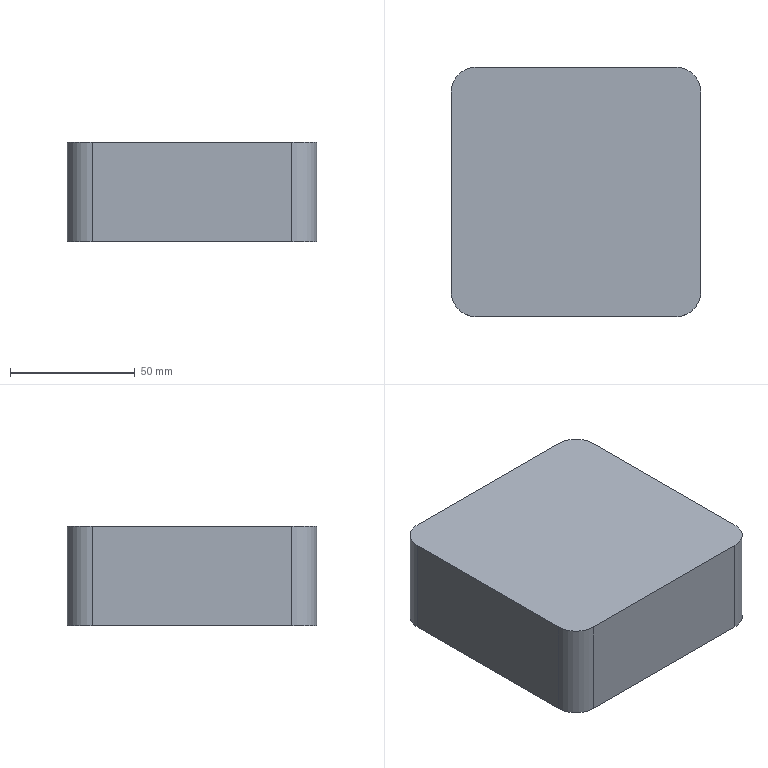Part | SolidWorks | features Extrusion 1, Fillet 1, ICE 1 | 1 solid | 13 faces | box 100 x 100 x 40 mm | volume 264030 mm3 | plane 7 | cylinder 6 | commonest cylinder face diameters 20 x4 75 x2
STEP:
#1=CARTESIAN_POINT('',(37.5,0.,30.));
#2=VERTEX_POINT('',#1);
#3=CARTESIAN_POINT('',(-37.5,0.,30.));
#4=VERTEX_POINT('',#3);
#5=CARTESIAN_POINT('',(0.,0.,30.));
#6=DIRECTION('',(0.,0.,-1.));
#7=DIRECTION('',(-1.,0.,0.));
#8=AXIS2_PLACEMENT_3D('',#5,#6,#7);
#9=CIRCLE('',#8,37.5);
#10=EDGE_CURVE('',#2,#4,#9,.T.);
#11=ORIENTED_EDGE('',*,*,#10,.F.);
#12=CARTESIAN_POINT('',(37.5,0.,0.));
#13=VERTEX_POINT('',#12);
#14=CARTESIAN_POINT('',(37.5,0.,30.));
#15=DIRECTION('',(0.,0.,-1.));
#16=VECTOR('',#15,1000.);
#17=LINE('',#14,#16);
#18=EDGE_CURVE('',#2,#13,#17,.T.);
#19=ORIENTED_EDGE('',*,*,#18,.T.);
#20=CARTESIAN_POINT('',(-37.5,0.,0.));
#21=VERTEX_POINT('',#20);
#22=CARTESIAN_POINT('',(0.,0.,0.));
#23=DIRECTION('',(0.,0.,-1.));
#24=DIRECTION('',(-1.,0.,0.));
#25=AXIS2_PLACEMENT_3D('',#22,#23,#24);
#26=CIRCLE('',#25,37.5);
#27=EDGE_CURVE('',#13,#21,#26,.T.);
#28=ORIENTED_EDGE('',*,*,#27,.T.);
#29=CARTESIAN_POINT('',(-37.5,0.,30.));
#30=DIRECTION('',(0.,0.,-1.));
#31=VECTOR('',#30,1000.);
#32=LINE('',#29,#31);
#33=EDGE_CURVE('',#4,#21,#32,.T.);
#34=ORIENTED_EDGE('',*,*,#33,.F.);
#35=EDGE_LOOP('',(#11,#19,#28,#34));
#36=FACE_OUTER_BOUND('',#35,.T.);
#37=CARTESIAN_POINT('',(0.,0.,30.));
#38=DIRECTION('',(0.,0.,-1.));
#39=DIRECTION('',(-1.,0.,0.));
#40=AXIS2_PLACEMENT_3D('',#37,#38,#39);
#41=CYLINDRICAL_SURFACE('',#40,37.5);
#42=ADVANCED_FACE('',(#36),#41,.F.);
#43=CARTESIAN_POINT('',(-40.,-50.,0.));
#44=VERTEX_POINT('',#43);
#45=CARTESIAN_POINT('',(40.,-50.,0.));
#46=VERTEX_POINT('',#45);
#47=CARTESIAN_POINT('',(-50.,-50.,0.));
#48=DIRECTION('',(1.,0.,0.));
#49=VECTOR('',#48,1000.);
#50=LINE('',#47,#49);
#51=EDGE_CURVE('',#44,#46,#50,.T.);
#52=ORIENTED_EDGE('',*,*,#51,.T.);
#53=CARTESIAN_POINT('',(40.,-50.,40.));
#54=VERTEX_POINT('',#53);
#55=CARTESIAN_POINT('',(40.,-50.,40.));
#56=DIRECTION('',(0.,0.,1.));
#57=VECTOR('',#56,1000.);
#58=LINE('',#55,#57);
#59=EDGE_CURVE('',#46,#54,#58,.T.);
#60=ORIENTED_EDGE('',*,*,#59,.T.);
#61=CARTESIAN_POINT('',(-40.,-50.,40.));
#62=VERTEX_POINT('',#61);
#63=CARTESIAN_POINT('',(-50.,-50.,40.));
#64=DIRECTION('',(1.,0.,0.));
#65=VECTOR('',#64,1000.);
#66=LINE('',#63,#65);
#67=EDGE_CURVE('',#62,#54,#66,.T.);
#68=ORIENTED_EDGE('',*,*,#67,.F.);
#69=CARTESIAN_POINT('',(-40.,-50.,0.));
#70=DIRECTION('',(0.,0.,-1.));
#71=VECTOR('',#70,1000.);
#72=LINE('',#69,#71);
#73=EDGE_CURVE('',#62,#44,#72,.T.);
#74=ORIENTED_EDGE('',*,*,#73,.T.);
#75=EDGE_LOOP('',(#52,#60,#68,#74));
#76=FACE_OUTER_BOUND('',#75,.T.);
#77=CARTESIAN_POINT('',(-50.,-50.,40.));
#78=DIRECTION('',(0.,1.,0.));
#79=DIRECTION('',(0.,0.,1.));
#80=AXIS2_PLACEMENT_3D('',#77,#78,#79);
#81=PLANE('',#80);
#82=ADVANCED_FACE('',(#76),#81,.F.);
#83=CARTESIAN_POINT('',(50.,-40.,40.));
#84=VERTEX_POINT('',#83);
#85=CARTESIAN_POINT('',(50.,40.,40.));
#86=VERTEX_POINT('',#85);
#87=CARTESIAN_POINT('',(50.,-50.,40.));
#88=DIRECTION('',(0.,1.,0.));
#89=VECTOR('',#88,1000.);
#90=LINE('',#87,#89);
#91=EDGE_CURVE('',#84,#86,#90,.T.);
#92=ORIENTED_EDGE('',*,*,#91,.F.);
#93=CARTESIAN_POINT('',(50.,-40.,0.));
#94=VERTEX_POINT('',#93);
#95=CARTESIAN_POINT('',(50.,-40.,40.));
#96=DIRECTION('',(0.,0.,-1.));
#97=VECTOR('',#96,1000.);
#98=LINE('',#95,#97);
#99=EDGE_CURVE('',#84,#94,#98,.T.);
#100=ORIENTED_EDGE('',*,*,#99,.T.);
#101=CARTESIAN_POINT('',(50.,40.,0.));
#102=VERTEX_POINT('',#101);
#103=CARTESIAN_POINT('',(50.,-50.,0.));
#104=DIRECTION('',(0.,1.,0.));
#105=VECTOR('',#104,1000.);
#106=LINE('',#103,#105);
#107=EDGE_CURVE('',#94,#102,#106,.T.);
#108=ORIENTED_EDGE('',*,*,#107,.T.);
#109=CARTESIAN_POINT('',(50.,40.,40.));
#110=DIRECTION('',(0.,0.,1.));
#111=VECTOR('',#110,1000.);
#112=LINE('',#109,#111);
#113=EDGE_CURVE('',#102,#86,#112,.T.);
#114=ORIENTED_EDGE('',*,*,#113,.T.);
#115=EDGE_LOOP('',(#92,#100,#108,#114));
#116=FACE_OUTER_BOUND('',#115,.T.);
#117=CARTESIAN_POINT('',(50.,-50.,40.));
#118=DIRECTION('',(-1.,0.,0.));
#119=DIRECTION('',(0.,0.,1.));
#120=AXIS2_PLACEMENT_3D('',#117,#118,#119);
#121=PLANE('',#120);
#122=ADVANCED_FACE('',(#116),#121,.F.);
#123=CARTESIAN_POINT('',(-40.,50.,40.));
#124=VERTEX_POINT('',#123);
#125=CARTESIAN_POINT('',(40.,50.,40.));
#126=VERTEX_POINT('',#125);
#127=CARTESIAN_POINT('',(-50.,50.,40.));
#128=DIRECTION('',(1.,0.,0.));
#129=VECTOR('',#128,1000.);
#130=LINE('',#127,#129);
#131=EDGE_CURVE('',#124,#126,#130,.T.);
#132=ORIENTED_EDGE('',*,*,#131,.T.);
#133=CARTESIAN_POINT('',(40.,50.,0.));
#134=VERTEX_POINT('',#133);
#135=CARTESIAN_POINT('',(40.,50.,0.));
#136=DIRECTION('',(0.,0.,-1.));
#137=VECTOR('',#136,1000.);
#138=LINE('',#135,#137);
#139=EDGE_CURVE('',#126,#134,#138,.T.);
#140=ORIENTED_EDGE('',*,*,#139,.T.);
#141=CARTESIAN_POINT('',(-40.,50.,0.));
#142=VERTEX_POINT('',#141);
#143=CARTESIAN_POINT('',(-50.,50.,0.));
#144=DIRECTION('',(1.,0.,0.));
#145=VECTOR('',#144,1000.);
#146=LINE('',#143,#145);
#147=EDGE_CURVE('',#142,#134,#146,.T.);
#148=ORIENTED_EDGE('',*,*,#147,.F.);
#149=CARTESIAN_POINT('',(-40.,50.,40.));
#150=DIRECTION('',(0.,0.,1.));
#151=VECTOR('',#150,1000.);
#152=LINE('',#149,#151);
#153=EDGE_CURVE('',#142,#124,#152,.T.);
#154=ORIENTED_EDGE('',*,*,#153,.T.);
#155=EDGE_LOOP('',(#132,#140,#148,#154));
#156=FACE_OUTER_BOUND('',#155,.T.);
#157=CARTESIAN_POINT('',(-50.,50.,40.));
#158=DIRECTION('',(0.,1.,0.));
#159=DIRECTION('',(0.,0.,1.));
#160=AXIS2_PLACEMENT_3D('',#157,#158,#159);
#161=PLANE('',#160);
#162=ADVANCED_FACE('',(#156),#161,.T.);
#163=CARTESIAN_POINT('',(-50.,-40.,0.));
#164=VERTEX_POINT('',#163);
#165=CARTESIAN_POINT('',(-50.,40.,0.));
#166=VERTEX_POINT('',#165);
#167=CARTESIAN_POINT('',(-50.,-50.,0.));
#168=DIRECTION('',(0.,1.,0.));
#169=VECTOR('',#168,1000.);
#170=LINE('',#167,#169);
#171=EDGE_CURVE('',#164,#166,#170,.T.);
#172=ORIENTED_EDGE('',*,*,#171,.F.);
#173=CARTESIAN_POINT('',(-50.,-40.,40.));
#174=VERTEX_POINT('',#173);
#175=CARTESIAN_POINT('',(-50.,-40.,40.));
#176=DIRECTION('',(0.,0.,1.));
#177=VECTOR('',#176,1000.);
#178=LINE('',#175,#177);
#179=EDGE_CURVE('',#164,#174,#178,.T.);
#180=ORIENTED_EDGE('',*,*,#179,.T.);
#181=CARTESIAN_POINT('',(-50.,40.,40.));
#182=VERTEX_POINT('',#181);
#183=CARTESIAN_POINT('',(-50.,-50.,40.));
#184=DIRECTION('',(0.,1.,0.));
#185=VECTOR('',#184,1000.);
#186=LINE('',#183,#185);
#187=EDGE_CURVE('',#174,#182,#186,.T.);
#188=ORIENTED_EDGE('',*,*,#187,.T.);
#189=CARTESIAN_POINT('',(-50.,40.,40.));
#190=DIRECTION('',(0.,0.,-1.));
#191=VECTOR('',#190,1000.);
#192=LINE('',#189,#191);
#193=EDGE_CURVE('',#182,#166,#192,.T.);
#194=ORIENTED_EDGE('',*,*,#193,.T.);
#195=EDGE_LOOP('',(#172,#180,#188,#194));
#196=FACE_OUTER_BOUND('',#195,.T.);
#197=CARTESIAN_POINT('',(-50.,-50.,40.));
#198=DIRECTION('',(-1.,0.,0.));
#199=DIRECTION('',(0.,0.,1.));
#200=AXIS2_PLACEMENT_3D('',#197,#198,#199);
#201=PLANE('',#200);
#202=ADVANCED_FACE('',(#196),#201,.T.);
#203=ORIENTED_EDGE('',*,*,#67,.T.);
#204=CARTESIAN_POINT('',(40.,-40.,40.));
#205=DIRECTION('',(0.,0.,1.));
#206=DIRECTION('',(1.,0.,0.));
#207=AXIS2_PLACEMENT_3D('',#204,#205,#206);
#208=CIRCLE('',#207,10.);
#209=EDGE_CURVE('',#54,#84,#208,.T.);
#210=ORIENTED_EDGE('',*,*,#209,.T.);
#211=ORIENTED_EDGE('',*,*,#91,.T.);
#212=CARTESIAN_POINT('',(40.,40.,40.));
#213=DIRECTION('',(0.,0.,1.));
#214=DIRECTION('',(1.,0.,0.));
#215=AXIS2_PLACEMENT_3D('',#212,#213,#214);
#216=CIRCLE('',#215,10.);
#217=EDGE_CURVE('',#86,#126,#216,.T.);
#218=ORIENTED_EDGE('',*,*,#217,.T.);
#219=ORIENTED_EDGE('',*,*,#131,.F.);
#220=CARTESIAN_POINT('',(-40.,40.,40.));
#221=DIRECTION('',(0.,0.,1.));
#222=DIRECTION('',(1.,0.,0.));
#223=AXIS2_PLACEMENT_3D('',#220,#221,#222);
#224=CIRCLE('',#223,10.);
#225=EDGE_CURVE('',#124,#182,#224,.T.);
#226=ORIENTED_EDGE('',*,*,#225,.T.);
#227=ORIENTED_EDGE('',*,*,#187,.F.);
#228=CARTESIAN_POINT('',(-40.,-40.,40.));
#229=DIRECTION('',(0.,0.,1.));
#230=DIRECTION('',(1.,0.,0.));
#231=AXIS2_PLACEMENT_3D('',#228,#229,#230);
#232=CIRCLE('',#231,10.);
#233=EDGE_CURVE('',#174,#62,#232,.T.);
#234=ORIENTED_EDGE('',*,*,#233,.T.);
#235=EDGE_LOOP('',(#203,#210,#211,#218,#219,#226,#227,#234));
#236=FACE_OUTER_BOUND('',#235,.T.);
#237=CARTESIAN_POINT('',(0.,0.,40.));
#238=DIRECTION('',(0.,0.,1.));
#239=DIRECTION('',(1.,0.,0.));
#240=AXIS2_PLACEMENT_3D('',#237,#238,#239);
#241=PLANE('',#240);
#242=ADVANCED_FACE('',(#236),#241,.T.);
#243=CARTESIAN_POINT('',(0.,0.,0.));
#244=DIRECTION('',(0.,0.,-1.));
#245=DIRECTION('',(-1.,0.,0.));
#246=AXIS2_PLACEMENT_3D('',#243,#244,#245);
#247=CIRCLE('',#246,37.5);
#248=EDGE_CURVE('',#21,#13,#247,.T.);
#249=ORIENTED_EDGE('',*,*,#248,.F.);
#250=ORIENTED_EDGE('',*,*,#27,.F.);
#251=EDGE_LOOP('',(#249,#250));
#252=FACE_BOUND('',#251,.T.);
#253=ORIENTED_EDGE('',*,*,#107,.F.);
#254=CARTESIAN_POINT('',(40.,-40.,0.));
#255=DIRECTION('',(0.,0.,-1.));
#256=DIRECTION('',(1.,0.,0.));
#257=AXIS2_PLACEMENT_3D('',#254,#255,#256);
#258=CIRCLE('',#257,10.);
#259=EDGE_CURVE('',#94,#46,#258,.T.);
#260=ORIENTED_EDGE('',*,*,#259,.T.);
#261=ORIENTED_EDGE('',*,*,#51,.F.);
#262=CARTESIAN_POINT('',(-40.,-40.,0.));
#263=DIRECTION('',(0.,0.,-1.));
#264=DIRECTION('',(1.,0.,0.));
#265=AXIS2_PLACEMENT_3D('',#262,#263,#264);
#266=CIRCLE('',#265,10.);
#267=EDGE_CURVE('',#44,#164,#266,.T.);
#268=ORIENTED_EDGE('',*,*,#267,.T.);
#269=ORIENTED_EDGE('',*,*,#171,.T.);
#270=CARTESIAN_POINT('',(-40.,40.,0.));
#271=DIRECTION('',(0.,0.,-1.));
#272=DIRECTION('',(1.,0.,0.));
#273=AXIS2_PLACEMENT_3D('',#270,#271,#272);
#274=CIRCLE('',#273,10.);
#275=EDGE_CURVE('',#166,#142,#274,.T.);
#276=ORIENTED_EDGE('',*,*,#275,.T.);
#277=ORIENTED_EDGE('',*,*,#147,.T.);
#278=CARTESIAN_POINT('',(40.,40.,0.));
#279=DIRECTION('',(0.,0.,-1.));
#280=DIRECTION('',(1.,0.,0.));
#281=AXIS2_PLACEMENT_3D('',#278,#279,#280);
#282=CIRCLE('',#281,10.);
#283=EDGE_CURVE('',#134,#102,#282,.T.);
#284=ORIENTED_EDGE('',*,*,#283,.T.);
#285=EDGE_LOOP('',(#253,#260,#261,#268,#269,#276,#277,#284));
#286=FACE_OUTER_BOUND('',#285,.T.);
#287=CARTESIAN_POINT('',(0.,0.,0.));
#288=DIRECTION('',(0.,0.,1.));
#289=DIRECTION('',(1.,0.,0.));
#290=AXIS2_PLACEMENT_3D('',#287,#288,#289);
#291=PLANE('',#290);
#292=ADVANCED_FACE('',(#252,#286),#291,.F.);
#293=ORIENTED_EDGE('',*,*,#18,.F.);
#294=CARTESIAN_POINT('',(0.,0.,30.));
#295=DIRECTION('',(0.,0.,-1.));
#296=DIRECTION('',(-1.,0.,0.));
#297=AXIS2_PLACEMENT_3D('',#294,#295,#296);
#298=CIRCLE('',#297,37.5);
#299=EDGE_CURVE('',#4,#2,#298,.T.);
#300=ORIENTED_EDGE('',*,*,#299,.F.);
#301=ORIENTED_EDGE('',*,*,#33,.T.);
#302=ORIENTED_EDGE('',*,*,#248,.T.);
#303=EDGE_LOOP('',(#293,#300,#301,#302));
#304=FACE_OUTER_BOUND('',#303,.T.);
#305=CARTESIAN_POINT('',(0.,0.,30.));
#306=DIRECTION('',(0.,0.,-1.));
#307=DIRECTION('',(-1.,0.,0.));
#308=AXIS2_PLACEMENT_3D('',#305,#306,#307);
#309=CYLINDRICAL_SURFACE('',#308,37.5);
#310=ADVANCED_FACE('',(#304),#309,.F.);
#311=ORIENTED_EDGE('',*,*,#299,.T.);
#312=ORIENTED_EDGE('',*,*,#10,.T.);
#313=EDGE_LOOP('',(#311,#312));
#314=FACE_OUTER_BOUND('',#313,.T.);
#315=CARTESIAN_POINT('',(0.,0.,30.));
#316=DIRECTION('',(0.,0.,-1.));
#317=DIRECTION('',(-1.,0.,0.));
#318=AXIS2_PLACEMENT_3D('',#315,#316,#317);
#319=PLANE('',#318);
#320=ADVANCED_FACE('',(#314),#319,.T.);
#321=ORIENTED_EDGE('',*,*,#209,.F.);
#322=ORIENTED_EDGE('',*,*,#59,.F.);
#323=ORIENTED_EDGE('',*,*,#259,.F.);
#324=ORIENTED_EDGE('',*,*,#99,.F.);
#325=EDGE_LOOP('',(#321,#322,#323,#324));
#326=FACE_OUTER_BOUND('',#325,.T.);
#327=CARTESIAN_POINT('',(40.,-40.,40.));
#328=DIRECTION('',(0.,0.,-1.));
#329=DIRECTION('',(-1.,0.,0.));
#330=AXIS2_PLACEMENT_3D('',#327,#328,#329);
#331=CYLINDRICAL_SURFACE('',#330,10.);
#332=ADVANCED_FACE('',(#326),#331,.T.);
#333=ORIENTED_EDGE('',*,*,#233,.F.);
#334=ORIENTED_EDGE('',*,*,#179,.F.);
#335=ORIENTED_EDGE('',*,*,#267,.F.);
#336=ORIENTED_EDGE('',*,*,#73,.F.);
#337=EDGE_LOOP('',(#333,#334,#335,#336));
#338=FACE_OUTER_BOUND('',#337,.T.);
#339=CARTESIAN_POINT('',(-40.,-40.,40.));
#340=DIRECTION('',(0.,0.,1.));
#341=DIRECTION('',(1.,0.,0.));
#342=AXIS2_PLACEMENT_3D('',#339,#340,#341);
#343=CYLINDRICAL_SURFACE('',#342,10.);
#344=ADVANCED_FACE('',(#338),#343,.T.);
#345=ORIENTED_EDGE('',*,*,#217,.F.);
#346=ORIENTED_EDGE('',*,*,#113,.F.);
#347=ORIENTED_EDGE('',*,*,#283,.F.);
#348=ORIENTED_EDGE('',*,*,#139,.F.);
#349=EDGE_LOOP('',(#345,#346,#347,#348));
#350=FACE_OUTER_BOUND('',#349,.T.);
#351=CARTESIAN_POINT('',(40.,40.,40.));
#352=DIRECTION('',(0.,0.,1.));
#353=DIRECTION('',(1.,0.,0.));
#354=AXIS2_PLACEMENT_3D('',#351,#352,#353);
#355=CYLINDRICAL_SURFACE('',#354,10.);
#356=ADVANCED_FACE('',(#350),#355,.T.);
#357=ORIENTED_EDGE('',*,*,#225,.F.);
#358=ORIENTED_EDGE('',*,*,#153,.F.);
#359=ORIENTED_EDGE('',*,*,#275,.F.);
#360=ORIENTED_EDGE('',*,*,#193,.F.);
#361=EDGE_LOOP('',(#357,#358,#359,#360));
#362=FACE_OUTER_BOUND('',#361,.T.);
#363=CARTESIAN_POINT('',(-40.,40.,40.));
#364=DIRECTION('',(0.,0.,-1.));
#365=DIRECTION('',(-1.,0.,0.));
#366=AXIS2_PLACEMENT_3D('',#363,#364,#365);
#367=CYLINDRICAL_SURFACE('',#366,10.);
#368=ADVANCED_FACE('',(#362),#367,.T.);
#369=CLOSED_SHELL('',(#42,#82,#122,#162,#202,#242,#292,#310,#320,#332,#344,#356,#368));
#370=MANIFOLD_SOLID_BREP('',#369);
#371=CARTESIAN_POINT('',(0.,0.,0.));
#372=DIRECTION('',(0.,0.,1.));
#373=DIRECTION('',(1.,0.,0.));
#374=AXIS2_PLACEMENT_3D('',#371,#372,#373);
#375=(LENGTH_UNIT()NAMED_UNIT(*)SI_UNIT(.MILLI.,.METRE.));
#376=UNCERTAINTY_MEASURE_WITH_UNIT(LENGTH_MEASURE(0.00001),#375,'','');
#377=(NAMED_UNIT(*)PLANE_ANGLE_UNIT()SI_UNIT($,.RADIAN.));
#378=(NAMED_UNIT(*)SI_UNIT($,.STERADIAN.)SOLID_ANGLE_UNIT());
#379=(GEOMETRIC_REPRESENTATION_CONTEXT(3)GLOBAL_UNCERTAINTY_ASSIGNED_CONTEXT((#376))GLOBAL_UNIT_ASSIGNED_CONTEXT((#375,#377,#378))REPRESENTATION_CONTEXT('',''));
#380=ADVANCED_BREP_SHAPE_REPRESENTATION('',(#370,#374),#379);